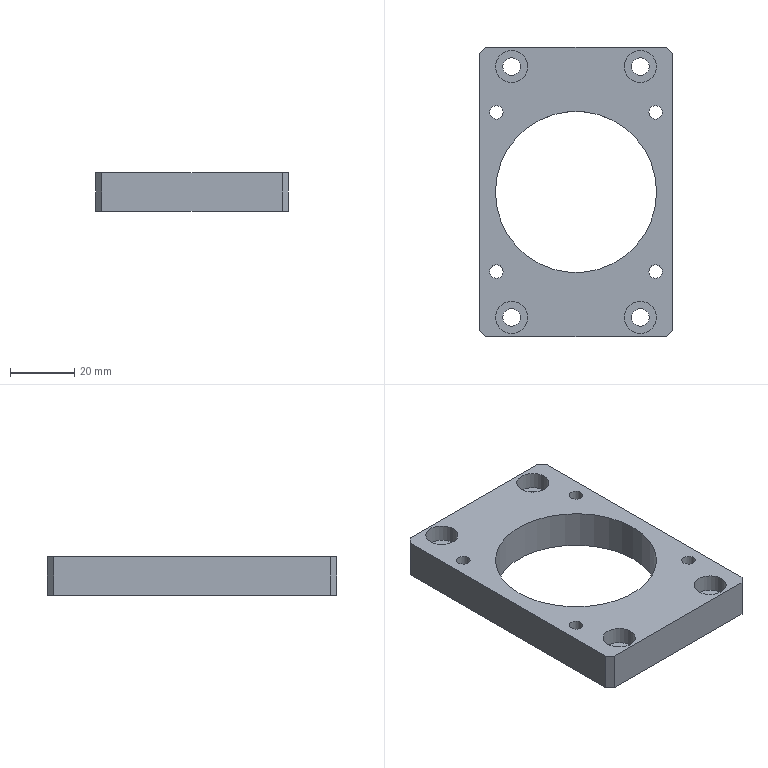Part | NX | 1 solid | 27 faces | box 60 x 90 x 12 mm | volume 38059 mm3 | plane 14 | cylinder 13 | commonest cylinder face diameters 4.2 x4 5.5 x4 10 x4 50.1 x1
STEP:
#1=CARTESIAN_POINT('',(-28.,45.,6.));
#2=VERTEX_POINT('',#1);
#3=CARTESIAN_POINT('',(-30.,43.,6.));
#4=VERTEX_POINT('',#3);
#5=CARTESIAN_POINT('',(-36.5,36.5,6.));
#6=DIRECTION('',(-0.7071,-0.7071,0.));
#7=VECTOR('',#6,1000.);
#8=LINE('',#5,#7);
#9=EDGE_CURVE('',#2,#4,#8,.T.);
#10=ORIENTED_EDGE('',*,*,#9,.F.);
#11=CARTESIAN_POINT('',(-28.,45.,-6.));
#12=VERTEX_POINT('',#11);
#13=CARTESIAN_POINT('',(-28.,45.,6.));
#14=DIRECTION('',(0.,0.,1.));
#15=VECTOR('',#14,1000.);
#16=LINE('',#13,#15);
#17=EDGE_CURVE('',#12,#2,#16,.T.);
#18=ORIENTED_EDGE('',*,*,#17,.F.);
#19=CARTESIAN_POINT('',(-30.,43.,-6.));
#20=VERTEX_POINT('',#19);
#21=CARTESIAN_POINT('',(-30.,43.,-6.));
#22=DIRECTION('',(0.7071,0.7071,0.));
#23=VECTOR('',#22,1000.);
#24=LINE('',#21,#23);
#25=EDGE_CURVE('',#20,#12,#24,.T.);
#26=ORIENTED_EDGE('',*,*,#25,.F.);
#27=CARTESIAN_POINT('',(-30.,43.,6.));
#28=DIRECTION('',(0.,0.,-1.));
#29=VECTOR('',#28,1000.);
#30=LINE('',#27,#29);
#31=EDGE_CURVE('',#4,#20,#30,.T.);
#32=ORIENTED_EDGE('',*,*,#31,.F.);
#33=EDGE_LOOP('',(#10,#18,#26,#32));
#34=FACE_BOUND('',#33,.T.);
#35=CARTESIAN_POINT('',(-30.,43.,6.));
#36=DIRECTION('',(0.7071,-0.7071,0.));
#37=DIRECTION('',(0.,0.,-1.));
#38=AXIS2_PLACEMENT_3D('',#35,#36,#37);
#39=PLANE('',#38);
#40=ADVANCED_FACE('',(#34),#39,.F.);
#41=CARTESIAN_POINT('',(-30.,-43.,6.));
#42=VERTEX_POINT('',#41);
#43=CARTESIAN_POINT('',(-28.,-45.,6.));
#44=VERTEX_POINT('',#43);
#45=CARTESIAN_POINT('',(-36.5,-36.5,6.));
#46=DIRECTION('',(0.7071,-0.7071,0.));
#47=VECTOR('',#46,1000.);
#48=LINE('',#45,#47);
#49=EDGE_CURVE('',#42,#44,#48,.T.);
#50=ORIENTED_EDGE('',*,*,#49,.F.);
#51=CARTESIAN_POINT('',(-30.,-43.,-6.));
#52=VERTEX_POINT('',#51);
#53=CARTESIAN_POINT('',(-30.,-43.,6.));
#54=DIRECTION('',(0.,0.,1.));
#55=VECTOR('',#54,1000.);
#56=LINE('',#53,#55);
#57=EDGE_CURVE('',#52,#42,#56,.T.);
#58=ORIENTED_EDGE('',*,*,#57,.F.);
#59=CARTESIAN_POINT('',(-28.,-45.,-6.));
#60=VERTEX_POINT('',#59);
#61=CARTESIAN_POINT('',(-28.,-45.,-6.));
#62=DIRECTION('',(-0.7071,0.7071,0.));
#63=VECTOR('',#62,1000.);
#64=LINE('',#61,#63);
#65=EDGE_CURVE('',#60,#52,#64,.T.);
#66=ORIENTED_EDGE('',*,*,#65,.F.);
#67=CARTESIAN_POINT('',(-28.,-45.,6.));
#68=DIRECTION('',(0.,0.,-1.));
#69=VECTOR('',#68,1000.);
#70=LINE('',#67,#69);
#71=EDGE_CURVE('',#44,#60,#70,.T.);
#72=ORIENTED_EDGE('',*,*,#71,.F.);
#73=EDGE_LOOP('',(#50,#58,#66,#72));
#74=FACE_BOUND('',#73,.T.);
#75=CARTESIAN_POINT('',(-28.,-45.,6.));
#76=DIRECTION('',(0.7071,0.7071,0.));
#77=DIRECTION('',(0.,0.,-1.));
#78=AXIS2_PLACEMENT_3D('',#75,#76,#77);
#79=PLANE('',#78);
#80=ADVANCED_FACE('',(#74),#79,.F.);
#81=CARTESIAN_POINT('',(28.,-45.,6.));
#82=VERTEX_POINT('',#81);
#83=CARTESIAN_POINT('',(30.,-43.,6.));
#84=VERTEX_POINT('',#83);
#85=CARTESIAN_POINT('',(36.5,-36.5,6.));
#86=DIRECTION('',(0.7071,0.7071,0.));
#87=VECTOR('',#86,1000.);
#88=LINE('',#85,#87);
#89=EDGE_CURVE('',#82,#84,#88,.T.);
#90=ORIENTED_EDGE('',*,*,#89,.F.);
#91=CARTESIAN_POINT('',(28.,-45.,-6.));
#92=VERTEX_POINT('',#91);
#93=CARTESIAN_POINT('',(28.,-45.,6.));
#94=DIRECTION('',(0.,0.,1.));
#95=VECTOR('',#94,1000.);
#96=LINE('',#93,#95);
#97=EDGE_CURVE('',#92,#82,#96,.T.);
#98=ORIENTED_EDGE('',*,*,#97,.F.);
#99=CARTESIAN_POINT('',(30.,-43.,-6.));
#100=VERTEX_POINT('',#99);
#101=CARTESIAN_POINT('',(30.,-43.,-6.));
#102=DIRECTION('',(-0.7071,-0.7071,0.));
#103=VECTOR('',#102,1000.);
#104=LINE('',#101,#103);
#105=EDGE_CURVE('',#100,#92,#104,.T.);
#106=ORIENTED_EDGE('',*,*,#105,.F.);
#107=CARTESIAN_POINT('',(30.,-43.,6.));
#108=DIRECTION('',(0.,0.,-1.));
#109=VECTOR('',#108,1000.);
#110=LINE('',#107,#109);
#111=EDGE_CURVE('',#84,#100,#110,.T.);
#112=ORIENTED_EDGE('',*,*,#111,.F.);
#113=EDGE_LOOP('',(#90,#98,#106,#112));
#114=FACE_BOUND('',#113,.T.);
#115=CARTESIAN_POINT('',(30.,-43.,6.));
#116=DIRECTION('',(-0.7071,0.7071,0.));
#117=DIRECTION('',(0.,0.,-1.));
#118=AXIS2_PLACEMENT_3D('',#115,#116,#117);
#119=PLANE('',#118);
#120=ADVANCED_FACE('',(#114),#119,.F.);
#121=CARTESIAN_POINT('',(30.,43.,6.));
#122=VERTEX_POINT('',#121);
#123=CARTESIAN_POINT('',(28.,45.,6.));
#124=VERTEX_POINT('',#123);
#125=CARTESIAN_POINT('',(36.5,36.5,6.));
#126=DIRECTION('',(-0.7071,0.7071,0.));
#127=VECTOR('',#126,1000.);
#128=LINE('',#125,#127);
#129=EDGE_CURVE('',#122,#124,#128,.T.);
#130=ORIENTED_EDGE('',*,*,#129,.F.);
#131=CARTESIAN_POINT('',(30.,43.,-6.));
#132=VERTEX_POINT('',#131);
#133=CARTESIAN_POINT('',(30.,43.,6.));
#134=DIRECTION('',(0.,0.,1.));
#135=VECTOR('',#134,1000.);
#136=LINE('',#133,#135);
#137=EDGE_CURVE('',#132,#122,#136,.T.);
#138=ORIENTED_EDGE('',*,*,#137,.F.);
#139=CARTESIAN_POINT('',(28.,45.,-6.));
#140=VERTEX_POINT('',#139);
#141=CARTESIAN_POINT('',(28.,45.,-6.));
#142=DIRECTION('',(0.7071,-0.7071,0.));
#143=VECTOR('',#142,1000.);
#144=LINE('',#141,#143);
#145=EDGE_CURVE('',#140,#132,#144,.T.);
#146=ORIENTED_EDGE('',*,*,#145,.F.);
#147=CARTESIAN_POINT('',(28.,45.,6.));
#148=DIRECTION('',(0.,0.,-1.));
#149=VECTOR('',#148,1000.);
#150=LINE('',#147,#149);
#151=EDGE_CURVE('',#124,#140,#150,.T.);
#152=ORIENTED_EDGE('',*,*,#151,.F.);
#153=EDGE_LOOP('',(#130,#138,#146,#152));
#154=FACE_BOUND('',#153,.T.);
#155=CARTESIAN_POINT('',(28.,45.,6.));
#156=DIRECTION('',(-0.7071,-0.7071,0.));
#157=DIRECTION('',(0.,0.,-1.));
#158=AXIS2_PLACEMENT_3D('',#155,#156,#157);
#159=PLANE('',#158);
#160=ADVANCED_FACE('',(#154),#159,.F.);
#161=CARTESIAN_POINT('',(-15.,-39.,0.6));
#162=VERTEX_POINT('',#161);
#163=CARTESIAN_POINT('',(-20.,-39.,0.6));
#164=DIRECTION('',(0.,0.,1.));
#165=DIRECTION('',(1.,0.,0.));
#166=AXIS2_PLACEMENT_3D('',#163,#164,#165);
#167=CIRCLE('',#166,5.);
#168=EDGE_CURVE('',#162,#162,#167,.T.);
#169=ORIENTED_EDGE('',*,*,#168,.T.);
#170=EDGE_LOOP('',(#169));
#171=FACE_BOUND('',#170,.T.);
#172=CARTESIAN_POINT('',(-17.25,-39.,0.6));
#173=VERTEX_POINT('',#172);
#174=CARTESIAN_POINT('',(-20.,-39.,0.6));
#175=DIRECTION('',(0.,0.,1.));
#176=DIRECTION('',(1.,0.,0.));
#177=AXIS2_PLACEMENT_3D('',#174,#175,#176);
#178=CIRCLE('',#177,2.75);
#179=EDGE_CURVE('',#173,#173,#178,.T.);
#180=ORIENTED_EDGE('',*,*,#179,.F.);
#181=EDGE_LOOP('',(#180));
#182=FACE_BOUND('',#181,.T.);
#183=CARTESIAN_POINT('',(-17.25,-39.,0.6));
#184=DIRECTION('',(0.,0.,-1.));
#185=DIRECTION('',(-1.,0.,0.));
#186=AXIS2_PLACEMENT_3D('',#183,#184,#185);
#187=PLANE('',#186);
#188=ADVANCED_FACE('',(#171,#182),#187,.F.);
#189=CARTESIAN_POINT('',(15.,-39.,0.6));
#190=VERTEX_POINT('',#189);
#191=CARTESIAN_POINT('',(20.,-39.,0.6));
#192=DIRECTION('',(0.,0.,1.));
#193=DIRECTION('',(-1.,0.,0.));
#194=AXIS2_PLACEMENT_3D('',#191,#192,#193);
#195=CIRCLE('',#194,5.);
#196=EDGE_CURVE('',#190,#190,#195,.T.);
#197=ORIENTED_EDGE('',*,*,#196,.T.);
#198=EDGE_LOOP('',(#197));
#199=FACE_BOUND('',#198,.T.);
#200=CARTESIAN_POINT('',(17.25,-39.,0.6));
#201=VERTEX_POINT('',#200);
#202=CARTESIAN_POINT('',(20.,-39.,0.6));
#203=DIRECTION('',(0.,0.,1.));
#204=DIRECTION('',(-1.,0.,0.));
#205=AXIS2_PLACEMENT_3D('',#202,#203,#204);
#206=CIRCLE('',#205,2.75);
#207=EDGE_CURVE('',#201,#201,#206,.T.);
#208=ORIENTED_EDGE('',*,*,#207,.F.);
#209=EDGE_LOOP('',(#208));
#210=FACE_BOUND('',#209,.T.);
#211=CARTESIAN_POINT('',(-17.25,-39.,0.6));
#212=DIRECTION('',(0.,0.,-1.));
#213=DIRECTION('',(-1.,0.,0.));
#214=AXIS2_PLACEMENT_3D('',#211,#212,#213);
#215=PLANE('',#214);
#216=ADVANCED_FACE('',(#199,#210),#215,.F.);
#217=CARTESIAN_POINT('',(-25.,39.,0.6));
#218=VERTEX_POINT('',#217);
#219=CARTESIAN_POINT('',(-20.,39.,0.6));
#220=DIRECTION('',(0.,0.,1.));
#221=DIRECTION('',(-1.,0.,0.));
#222=AXIS2_PLACEMENT_3D('',#219,#220,#221);
#223=CIRCLE('',#222,5.);
#224=EDGE_CURVE('',#218,#218,#223,.T.);
#225=ORIENTED_EDGE('',*,*,#224,.T.);
#226=EDGE_LOOP('',(#225));
#227=FACE_BOUND('',#226,.T.);
#228=CARTESIAN_POINT('',(-22.75,39.,0.6));
#229=VERTEX_POINT('',#228);
#230=CARTESIAN_POINT('',(-20.,39.,0.6));
#231=DIRECTION('',(0.,0.,1.));
#232=DIRECTION('',(-1.,0.,0.));
#233=AXIS2_PLACEMENT_3D('',#230,#231,#232);
#234=CIRCLE('',#233,2.75);
#235=EDGE_CURVE('',#229,#229,#234,.T.);
#236=ORIENTED_EDGE('',*,*,#235,.F.);
#237=EDGE_LOOP('',(#236));
#238=FACE_BOUND('',#237,.T.);
#239=CARTESIAN_POINT('',(-17.25,-39.,0.6));
#240=DIRECTION('',(0.,0.,-1.));
#241=DIRECTION('',(-1.,0.,0.));
#242=AXIS2_PLACEMENT_3D('',#239,#240,#241);
#243=PLANE('',#242);
#244=ADVANCED_FACE('',(#227,#238),#243,.F.);
#245=CARTESIAN_POINT('',(15.,39.,0.6));
#246=VERTEX_POINT('',#245);
#247=CARTESIAN_POINT('',(20.,39.,0.6));
#248=DIRECTION('',(0.,0.,1.));
#249=DIRECTION('',(-1.,0.,0.));
#250=AXIS2_PLACEMENT_3D('',#247,#248,#249);
#251=CIRCLE('',#250,5.);
#252=EDGE_CURVE('',#246,#246,#251,.T.);
#253=ORIENTED_EDGE('',*,*,#252,.T.);
#254=EDGE_LOOP('',(#253));
#255=FACE_BOUND('',#254,.T.);
#256=CARTESIAN_POINT('',(17.25,39.,0.6));
#257=VERTEX_POINT('',#256);
#258=CARTESIAN_POINT('',(20.,39.,0.6));
#259=DIRECTION('',(0.,0.,1.));
#260=DIRECTION('',(-1.,0.,0.));
#261=AXIS2_PLACEMENT_3D('',#258,#259,#260);
#262=CIRCLE('',#261,2.75);
#263=EDGE_CURVE('',#257,#257,#262,.T.);
#264=ORIENTED_EDGE('',*,*,#263,.F.);
#265=EDGE_LOOP('',(#264));
#266=FACE_BOUND('',#265,.T.);
#267=CARTESIAN_POINT('',(-17.25,-39.,0.6));
#268=DIRECTION('',(0.,0.,-1.));
#269=DIRECTION('',(-1.,0.,0.));
#270=AXIS2_PLACEMENT_3D('',#267,#268,#269);
#271=PLANE('',#270);
#272=ADVANCED_FACE('',(#255,#266),#271,.F.);
#273=CARTESIAN_POINT('',(30.,45.,-6.));
#274=DIRECTION('',(-1.,0.,0.));
#275=VECTOR('',#274,1000.);
#276=LINE('',#273,#275);
#277=EDGE_CURVE('',#140,#12,#276,.T.);
#278=ORIENTED_EDGE('',*,*,#277,.F.);
#279=ORIENTED_EDGE('',*,*,#145,.T.);
#280=CARTESIAN_POINT('',(30.,-45.,-6.));
#281=DIRECTION('',(0.,1.,0.));
#282=VECTOR('',#281,1000.);
#283=LINE('',#280,#282);
#284=EDGE_CURVE('',#100,#132,#283,.T.);
#285=ORIENTED_EDGE('',*,*,#284,.F.);
#286=ORIENTED_EDGE('',*,*,#105,.T.);
#287=CARTESIAN_POINT('',(30.,-45.,-6.));
#288=DIRECTION('',(1.,0.,0.));
#289=VECTOR('',#288,1000.);
#290=LINE('',#287,#289);
#291=EDGE_CURVE('',#60,#92,#290,.T.);
#292=ORIENTED_EDGE('',*,*,#291,.F.);
#293=ORIENTED_EDGE('',*,*,#65,.T.);
#294=CARTESIAN_POINT('',(-30.,-45.,-6.));
#295=DIRECTION('',(0.,-1.,0.));
#296=VECTOR('',#295,1000.);
#297=LINE('',#294,#296);
#298=EDGE_CURVE('',#20,#52,#297,.T.);
#299=ORIENTED_EDGE('',*,*,#298,.F.);
#300=ORIENTED_EDGE('',*,*,#25,.T.);
#301=EDGE_LOOP('',(#278,#279,#285,#286,#292,#293,#299,#300));
#302=FACE_BOUND('',#301,.T.);
#303=CARTESIAN_POINT('',(26.849,24.749,-6.));
#304=VERTEX_POINT('',#303);
#305=CARTESIAN_POINT('',(24.749,24.749,-6.));
#306=DIRECTION('',(0.,0.,1.));
#307=DIRECTION('',(1.,0.,0.));
#308=AXIS2_PLACEMENT_3D('',#305,#306,#307);
#309=CIRCLE('',#308,2.1);
#310=EDGE_CURVE('',#304,#304,#309,.T.);
#311=ORIENTED_EDGE('',*,*,#310,.T.);
#312=EDGE_LOOP('',(#311));
#313=FACE_BOUND('',#312,.T.);
#314=CARTESIAN_POINT('',(26.849,-24.749,-6.));
#315=VERTEX_POINT('',#314);
#316=CARTESIAN_POINT('',(24.749,-24.749,-6.));
#317=DIRECTION('',(0.,0.,1.));
#318=DIRECTION('',(1.,0.,0.));
#319=AXIS2_PLACEMENT_3D('',#316,#317,#318);
#320=CIRCLE('',#319,2.1);
#321=EDGE_CURVE('',#315,#315,#320,.T.);
#322=ORIENTED_EDGE('',*,*,#321,.T.);
#323=EDGE_LOOP('',(#322));
#324=FACE_BOUND('',#323,.T.);
#325=CARTESIAN_POINT('',(-22.649,-24.749,-6.));
#326=VERTEX_POINT('',#325);
#327=CARTESIAN_POINT('',(-24.749,-24.749,-6.));
#328=DIRECTION('',(0.,0.,1.));
#329=DIRECTION('',(1.,0.,0.));
#330=AXIS2_PLACEMENT_3D('',#327,#328,#329);
#331=CIRCLE('',#330,2.1);
#332=EDGE_CURVE('',#326,#326,#331,.T.);
#333=ORIENTED_EDGE('',*,*,#332,.T.);
#334=EDGE_LOOP('',(#333));
#335=FACE_BOUND('',#334,.T.);
#336=CARTESIAN_POINT('',(-22.649,24.749,-6.));
#337=VERTEX_POINT('',#336);
#338=CARTESIAN_POINT('',(-24.749,24.749,-6.));
#339=DIRECTION('',(0.,0.,1.));
#340=DIRECTION('',(1.,0.,0.));
#341=AXIS2_PLACEMENT_3D('',#338,#339,#340);
#342=CIRCLE('',#341,2.1);
#343=EDGE_CURVE('',#337,#337,#342,.T.);
#344=ORIENTED_EDGE('',*,*,#343,.T.);
#345=EDGE_LOOP('',(#344));
#346=FACE_BOUND('',#345,.T.);
#347=CARTESIAN_POINT('',(25.05,0.,-6.));
#348=VERTEX_POINT('',#347);
#349=CARTESIAN_POINT('',(0.,0.,-6.));
#350=DIRECTION('',(0.,0.,1.));
#351=DIRECTION('',(1.,0.,0.));
#352=AXIS2_PLACEMENT_3D('',#349,#350,#351);
#353=CIRCLE('',#352,25.05);
#354=EDGE_CURVE('',#348,#348,#353,.T.);
#355=ORIENTED_EDGE('',*,*,#354,.T.);
#356=EDGE_LOOP('',(#355));
#357=FACE_BOUND('',#356,.T.);
#358=CARTESIAN_POINT('',(22.75,39.,-6.));
#359=VERTEX_POINT('',#358);
#360=CARTESIAN_POINT('',(20.,39.,-6.));
#361=DIRECTION('',(0.,0.,1.));
#362=DIRECTION('',(1.,0.,0.));
#363=AXIS2_PLACEMENT_3D('',#360,#361,#362);
#364=CIRCLE('',#363,2.75);
#365=EDGE_CURVE('',#359,#359,#364,.T.);
#366=ORIENTED_EDGE('',*,*,#365,.T.);
#367=EDGE_LOOP('',(#366));
#368=FACE_BOUND('',#367,.T.);
#369=CARTESIAN_POINT('',(-17.25,39.,-6.));
#370=VERTEX_POINT('',#369);
#371=CARTESIAN_POINT('',(-20.,39.,-6.));
#372=DIRECTION('',(0.,0.,1.));
#373=DIRECTION('',(1.,0.,0.));
#374=AXIS2_PLACEMENT_3D('',#371,#372,#373);
#375=CIRCLE('',#374,2.75);
#376=EDGE_CURVE('',#370,#370,#375,.T.);
#377=ORIENTED_EDGE('',*,*,#376,.T.);
#378=EDGE_LOOP('',(#377));
#379=FACE_BOUND('',#378,.T.);
#380=CARTESIAN_POINT('',(22.75,-39.,-6.));
#381=VERTEX_POINT('',#380);
#382=CARTESIAN_POINT('',(20.,-39.,-6.));
#383=DIRECTION('',(0.,0.,1.));
#384=DIRECTION('',(1.,0.,0.));
#385=AXIS2_PLACEMENT_3D('',#382,#383,#384);
#386=CIRCLE('',#385,2.75);
#387=EDGE_CURVE('',#381,#381,#386,.T.);
#388=ORIENTED_EDGE('',*,*,#387,.T.);
#389=EDGE_LOOP('',(#388));
#390=FACE_BOUND('',#389,.T.);
#391=CARTESIAN_POINT('',(-17.25,-39.,-6.));
#392=VERTEX_POINT('',#391);
#393=CARTESIAN_POINT('',(-20.,-39.,-6.));
#394=DIRECTION('',(0.,0.,1.));
#395=DIRECTION('',(1.,0.,0.));
#396=AXIS2_PLACEMENT_3D('',#393,#394,#395);
#397=CIRCLE('',#396,2.75);
#398=EDGE_CURVE('',#392,#392,#397,.T.);
#399=ORIENTED_EDGE('',*,*,#398,.T.);
#400=EDGE_LOOP('',(#399));
#401=FACE_BOUND('',#400,.T.);
#402=CARTESIAN_POINT('',(0.,0.,-6.));
#403=DIRECTION('',(0.,0.,1.));
#404=DIRECTION('',(1.,0.,0.));
#405=AXIS2_PLACEMENT_3D('',#402,#403,#404);
#406=PLANE('',#405);
#407=ADVANCED_FACE('',(#302,#313,#324,#335,#346,#357,#368,#379,#390,#401),#406,.F.);
#408=CARTESIAN_POINT('',(30.,-45.,6.));
#409=DIRECTION('',(0.,1.,0.));
#410=VECTOR('',#409,1000.);
#411=LINE('',#408,#410);
#412=EDGE_CURVE('',#84,#122,#411,.T.);
#413=ORIENTED_EDGE('',*,*,#412,.T.);
#414=ORIENTED_EDGE('',*,*,#129,.T.);
#415=CARTESIAN_POINT('',(30.,45.,6.));
#416=DIRECTION('',(-1.,0.,0.));
#417=VECTOR('',#416,1000.);
#418=LINE('',#415,#417);
#419=EDGE_CURVE('',#124,#2,#418,.T.);
#420=ORIENTED_EDGE('',*,*,#419,.T.);
#421=ORIENTED_EDGE('',*,*,#9,.T.);
#422=CARTESIAN_POINT('',(-30.,-45.,6.));
#423=DIRECTION('',(0.,-1.,0.));
#424=VECTOR('',#423,1000.);
#425=LINE('',#422,#424);
#426=EDGE_CURVE('',#4,#42,#425,.T.);
#427=ORIENTED_EDGE('',*,*,#426,.T.);
#428=ORIENTED_EDGE('',*,*,#49,.T.);
#429=CARTESIAN_POINT('',(30.,-45.,6.));
#430=DIRECTION('',(1.,0.,0.));
#431=VECTOR('',#430,1000.);
#432=LINE('',#429,#431);
#433=EDGE_CURVE('',#44,#82,#432,.T.);
#434=ORIENTED_EDGE('',*,*,#433,.T.);
#435=ORIENTED_EDGE('',*,*,#89,.T.);
#436=EDGE_LOOP('',(#413,#414,#420,#421,#427,#428,#434,#435));
#437=FACE_BOUND('',#436,.T.);
#438=CARTESIAN_POINT('',(26.849,24.749,6.));
#439=VERTEX_POINT('',#438);
#440=CARTESIAN_POINT('',(24.749,24.749,6.));
#441=DIRECTION('',(0.,0.,1.));
#442=DIRECTION('',(1.,0.,0.));
#443=AXIS2_PLACEMENT_3D('',#440,#441,#442);
#444=CIRCLE('',#443,2.1);
#445=EDGE_CURVE('',#439,#439,#444,.T.);
#446=ORIENTED_EDGE('',*,*,#445,.F.);
#447=EDGE_LOOP('',(#446));
#448=FACE_BOUND('',#447,.T.);
#449=CARTESIAN_POINT('',(26.849,-24.749,6.));
#450=VERTEX_POINT('',#449);
#451=CARTESIAN_POINT('',(24.749,-24.749,6.));
#452=DIRECTION('',(0.,0.,1.));
#453=DIRECTION('',(1.,0.,0.));
#454=AXIS2_PLACEMENT_3D('',#451,#452,#453);
#455=CIRCLE('',#454,2.1);
#456=EDGE_CURVE('',#450,#450,#455,.T.);
#457=ORIENTED_EDGE('',*,*,#456,.F.);
#458=EDGE_LOOP('',(#457));
#459=FACE_BOUND('',#458,.T.);
#460=CARTESIAN_POINT('',(-22.649,-24.749,6.));
#461=VERTEX_POINT('',#460);
#462=CARTESIAN_POINT('',(-24.749,-24.749,6.));
#463=DIRECTION('',(0.,0.,1.));
#464=DIRECTION('',(1.,0.,0.));
#465=AXIS2_PLACEMENT_3D('',#462,#463,#464);
#466=CIRCLE('',#465,2.1);
#467=EDGE_CURVE('',#461,#461,#466,.T.);
#468=ORIENTED_EDGE('',*,*,#467,.F.);
#469=EDGE_LOOP('',(#468));
#470=FACE_BOUND('',#469,.T.);
#471=CARTESIAN_POINT('',(-22.649,24.749,6.));
#472=VERTEX_POINT('',#471);
#473=CARTESIAN_POINT('',(-24.749,24.749,6.));
#474=DIRECTION('',(0.,0.,1.));
#475=DIRECTION('',(1.,0.,0.));
#476=AXIS2_PLACEMENT_3D('',#473,#474,#475);
#477=CIRCLE('',#476,2.1);
#478=EDGE_CURVE('',#472,#472,#477,.T.);
#479=ORIENTED_EDGE('',*,*,#478,.F.);
#480=EDGE_LOOP('',(#479));
#481=FACE_BOUND('',#480,.T.);
#482=CARTESIAN_POINT('',(25.05,0.,6.));
#483=VERTEX_POINT('',#482);
#484=CARTESIAN_POINT('',(0.,0.,6.));
#485=DIRECTION('',(0.,0.,1.));
#486=DIRECTION('',(1.,0.,0.));
#487=AXIS2_PLACEMENT_3D('',#484,#485,#486);
#488=CIRCLE('',#487,25.05);
#489=EDGE_CURVE('',#483,#483,#488,.T.);
#490=ORIENTED_EDGE('',*,*,#489,.F.);
#491=EDGE_LOOP('',(#490));
#492=FACE_BOUND('',#491,.T.);
#493=CARTESIAN_POINT('',(25.,39.,6.));
#494=VERTEX_POINT('',#493);
#495=CARTESIAN_POINT('',(20.,39.,6.));
#496=DIRECTION('',(0.,0.,1.));
#497=DIRECTION('',(1.,0.,0.));
#498=AXIS2_PLACEMENT_3D('',#495,#496,#497);
#499=CIRCLE('',#498,5.);
#500=EDGE_CURVE('',#494,#494,#499,.T.);
#501=ORIENTED_EDGE('',*,*,#500,.F.);
#502=EDGE_LOOP('',(#501));
#503=FACE_BOUND('',#502,.T.);
#504=CARTESIAN_POINT('',(-15.,39.,6.));
#505=VERTEX_POINT('',#504);
#506=CARTESIAN_POINT('',(-20.,39.,6.));
#507=DIRECTION('',(0.,0.,1.));
#508=DIRECTION('',(1.,0.,0.));
#509=AXIS2_PLACEMENT_3D('',#506,#507,#508);
#510=CIRCLE('',#509,5.);
#511=EDGE_CURVE('',#505,#505,#510,.T.);
#512=ORIENTED_EDGE('',*,*,#511,.F.);
#513=EDGE_LOOP('',(#512));
#514=FACE_BOUND('',#513,.T.);
#515=CARTESIAN_POINT('',(25.,-39.,6.));
#516=VERTEX_POINT('',#515);
#517=CARTESIAN_POINT('',(20.,-39.,6.));
#518=DIRECTION('',(0.,0.,1.));
#519=DIRECTION('',(1.,0.,0.));
#520=AXIS2_PLACEMENT_3D('',#517,#518,#519);
#521=CIRCLE('',#520,5.);
#522=EDGE_CURVE('',#516,#516,#521,.T.);
#523=ORIENTED_EDGE('',*,*,#522,.F.);
#524=EDGE_LOOP('',(#523));
#525=FACE_BOUND('',#524,.T.);
#526=CARTESIAN_POINT('',(-15.,-39.,6.));
#527=VERTEX_POINT('',#526);
#528=CARTESIAN_POINT('',(-20.,-39.,6.));
#529=DIRECTION('',(0.,0.,1.));
#530=DIRECTION('',(1.,0.,0.));
#531=AXIS2_PLACEMENT_3D('',#528,#529,#530);
#532=CIRCLE('',#531,5.);
#533=EDGE_CURVE('',#527,#527,#532,.T.);
#534=ORIENTED_EDGE('',*,*,#533,.F.);
#535=EDGE_LOOP('',(#534));
#536=FACE_BOUND('',#535,.T.);
#537=CARTESIAN_POINT('',(0.,0.,6.));
#538=DIRECTION('',(0.,0.,1.));
#539=DIRECTION('',(1.,0.,0.));
#540=AXIS2_PLACEMENT_3D('',#537,#538,#539);
#541=PLANE('',#540);
#542=ADVANCED_FACE('',(#437,#448,#459,#470,#481,#492,#503,#514,#525,#536),#541,.T.);
#543=ORIENTED_EDGE('',*,*,#419,.F.);
#544=ORIENTED_EDGE('',*,*,#151,.T.);
#545=ORIENTED_EDGE('',*,*,#277,.T.);
#546=ORIENTED_EDGE('',*,*,#17,.T.);
#547=EDGE_LOOP('',(#543,#544,#545,#546));
#548=FACE_BOUND('',#547,.T.);
#549=CARTESIAN_POINT('',(30.,45.,6.));
#550=DIRECTION('',(0.,-1.,0.));
#551=DIRECTION('',(1.,0.,0.));
#552=AXIS2_PLACEMENT_3D('',#549,#550,#551);
#553=PLANE('',#552);
#554=ADVANCED_FACE('',(#548),#553,.F.);
#555=ORIENTED_EDGE('',*,*,#284,.T.);
#556=ORIENTED_EDGE('',*,*,#137,.T.);
#557=ORIENTED_EDGE('',*,*,#412,.F.);
#558=ORIENTED_EDGE('',*,*,#111,.T.);
#559=EDGE_LOOP('',(#555,#556,#557,#558));
#560=FACE_BOUND('',#559,.T.);
#561=CARTESIAN_POINT('',(30.,-45.,6.));
#562=DIRECTION('',(-1.,0.,0.));
#563=DIRECTION('',(0.,-1.,0.));
#564=AXIS2_PLACEMENT_3D('',#561,#562,#563);
#565=PLANE('',#564);
#566=ADVANCED_FACE('',(#560),#565,.F.);
#567=ORIENTED_EDGE('',*,*,#291,.T.);
#568=ORIENTED_EDGE('',*,*,#97,.T.);
#569=ORIENTED_EDGE('',*,*,#433,.F.);
#570=ORIENTED_EDGE('',*,*,#71,.T.);
#571=EDGE_LOOP('',(#567,#568,#569,#570));
#572=FACE_BOUND('',#571,.T.);
#573=CARTESIAN_POINT('',(30.,-45.,6.));
#574=DIRECTION('',(0.,1.,0.));
#575=DIRECTION('',(-1.,0.,0.));
#576=AXIS2_PLACEMENT_3D('',#573,#574,#575);
#577=PLANE('',#576);
#578=ADVANCED_FACE('',(#572),#577,.F.);
#579=ORIENTED_EDGE('',*,*,#298,.T.);
#580=ORIENTED_EDGE('',*,*,#57,.T.);
#581=ORIENTED_EDGE('',*,*,#426,.F.);
#582=ORIENTED_EDGE('',*,*,#31,.T.);
#583=EDGE_LOOP('',(#579,#580,#581,#582));
#584=FACE_BOUND('',#583,.T.);
#585=CARTESIAN_POINT('',(-30.,-45.,6.));
#586=DIRECTION('',(1.,0.,0.));
#587=DIRECTION('',(0.,0.,-1.));
#588=AXIS2_PLACEMENT_3D('',#585,#586,#587);
#589=PLANE('',#588);
#590=ADVANCED_FACE('',(#584),#589,.F.);
#591=ORIENTED_EDGE('',*,*,#310,.F.);
#592=EDGE_LOOP('',(#591));
#593=FACE_BOUND('',#592,.T.);
#594=ORIENTED_EDGE('',*,*,#445,.T.);
#595=EDGE_LOOP('',(#594));
#596=FACE_BOUND('',#595,.T.);
#597=CARTESIAN_POINT('',(24.749,24.749,6.));
#598=DIRECTION('',(0.,0.,1.));
#599=DIRECTION('',(1.,0.,0.));
#600=AXIS2_PLACEMENT_3D('',#597,#598,#599);
#601=CYLINDRICAL_SURFACE('',#600,2.1);
#602=ADVANCED_FACE('',(#593,#596),#601,.F.);
#603=ORIENTED_EDGE('',*,*,#321,.F.);
#604=EDGE_LOOP('',(#603));
#605=FACE_BOUND('',#604,.T.);
#606=ORIENTED_EDGE('',*,*,#456,.T.);
#607=EDGE_LOOP('',(#606));
#608=FACE_BOUND('',#607,.T.);
#609=CARTESIAN_POINT('',(24.749,-24.749,6.));
#610=DIRECTION('',(0.,0.,1.));
#611=DIRECTION('',(1.,0.,0.));
#612=AXIS2_PLACEMENT_3D('',#609,#610,#611);
#613=CYLINDRICAL_SURFACE('',#612,2.1);
#614=ADVANCED_FACE('',(#605,#608),#613,.F.);
#615=ORIENTED_EDGE('',*,*,#332,.F.);
#616=EDGE_LOOP('',(#615));
#617=FACE_BOUND('',#616,.T.);
#618=ORIENTED_EDGE('',*,*,#467,.T.);
#619=EDGE_LOOP('',(#618));
#620=FACE_BOUND('',#619,.T.);
#621=CARTESIAN_POINT('',(-24.749,-24.749,6.));
#622=DIRECTION('',(0.,0.,1.));
#623=DIRECTION('',(1.,0.,0.));
#624=AXIS2_PLACEMENT_3D('',#621,#622,#623);
#625=CYLINDRICAL_SURFACE('',#624,2.1);
#626=ADVANCED_FACE('',(#617,#620),#625,.F.);
#627=ORIENTED_EDGE('',*,*,#343,.F.);
#628=EDGE_LOOP('',(#627));
#629=FACE_BOUND('',#628,.T.);
#630=ORIENTED_EDGE('',*,*,#478,.T.);
#631=EDGE_LOOP('',(#630));
#632=FACE_BOUND('',#631,.T.);
#633=CARTESIAN_POINT('',(-24.749,24.749,6.));
#634=DIRECTION('',(0.,0.,1.));
#635=DIRECTION('',(1.,0.,0.));
#636=AXIS2_PLACEMENT_3D('',#633,#634,#635);
#637=CYLINDRICAL_SURFACE('',#636,2.1);
#638=ADVANCED_FACE('',(#629,#632),#637,.F.);
#639=ORIENTED_EDGE('',*,*,#354,.F.);
#640=EDGE_LOOP('',(#639));
#641=FACE_BOUND('',#640,.T.);
#642=ORIENTED_EDGE('',*,*,#489,.T.);
#643=EDGE_LOOP('',(#642));
#644=FACE_BOUND('',#643,.T.);
#645=CARTESIAN_POINT('',(0.,0.,-6.));
#646=DIRECTION('',(0.,0.,1.));
#647=DIRECTION('',(1.,0.,0.));
#648=AXIS2_PLACEMENT_3D('',#645,#646,#647);
#649=CYLINDRICAL_SURFACE('',#648,25.05);
#650=ADVANCED_FACE('',(#641,#644),#649,.F.);
#651=ORIENTED_EDGE('',*,*,#365,.F.);
#652=EDGE_LOOP('',(#651));
#653=FACE_BOUND('',#652,.T.);
#654=ORIENTED_EDGE('',*,*,#263,.T.);
#655=EDGE_LOOP('',(#654));
#656=FACE_BOUND('',#655,.T.);
#657=CARTESIAN_POINT('',(20.,39.,6.));
#658=DIRECTION('',(0.,0.,1.));
#659=DIRECTION('',(1.,0.,0.));
#660=AXIS2_PLACEMENT_3D('',#657,#658,#659);
#661=CYLINDRICAL_SURFACE('',#660,2.75);
#662=ADVANCED_FACE('',(#653,#656),#661,.F.);
#663=ORIENTED_EDGE('',*,*,#252,.F.);
#664=EDGE_LOOP('',(#663));
#665=FACE_BOUND('',#664,.T.);
#666=ORIENTED_EDGE('',*,*,#500,.T.);
#667=EDGE_LOOP('',(#666));
#668=FACE_BOUND('',#667,.T.);
#669=CARTESIAN_POINT('',(20.,39.,6.));
#670=DIRECTION('',(0.,0.,1.));
#671=DIRECTION('',(1.,0.,0.));
#672=AXIS2_PLACEMENT_3D('',#669,#670,#671);
#673=CYLINDRICAL_SURFACE('',#672,5.);
#674=ADVANCED_FACE('',(#665,#668),#673,.F.);
#675=ORIENTED_EDGE('',*,*,#376,.F.);
#676=EDGE_LOOP('',(#675));
#677=FACE_BOUND('',#676,.T.);
#678=ORIENTED_EDGE('',*,*,#235,.T.);
#679=EDGE_LOOP('',(#678));
#680=FACE_BOUND('',#679,.T.);
#681=CARTESIAN_POINT('',(-20.,39.,6.));
#682=DIRECTION('',(0.,0.,1.));
#683=DIRECTION('',(1.,0.,0.));
#684=AXIS2_PLACEMENT_3D('',#681,#682,#683);
#685=CYLINDRICAL_SURFACE('',#684,2.75);
#686=ADVANCED_FACE('',(#677,#680),#685,.F.);
#687=ORIENTED_EDGE('',*,*,#224,.F.);
#688=EDGE_LOOP('',(#687));
#689=FACE_BOUND('',#688,.T.);
#690=ORIENTED_EDGE('',*,*,#511,.T.);
#691=EDGE_LOOP('',(#690));
#692=FACE_BOUND('',#691,.T.);
#693=CARTESIAN_POINT('',(-20.,39.,6.));
#694=DIRECTION('',(0.,0.,1.));
#695=DIRECTION('',(1.,0.,0.));
#696=AXIS2_PLACEMENT_3D('',#693,#694,#695);
#697=CYLINDRICAL_SURFACE('',#696,5.);
#698=ADVANCED_FACE('',(#689,#692),#697,.F.);
#699=ORIENTED_EDGE('',*,*,#387,.F.);
#700=EDGE_LOOP('',(#699));
#701=FACE_BOUND('',#700,.T.);
#702=ORIENTED_EDGE('',*,*,#207,.T.);
#703=EDGE_LOOP('',(#702));
#704=FACE_BOUND('',#703,.T.);
#705=CARTESIAN_POINT('',(20.,-39.,6.));
#706=DIRECTION('',(0.,0.,1.));
#707=DIRECTION('',(1.,0.,0.));
#708=AXIS2_PLACEMENT_3D('',#705,#706,#707);
#709=CYLINDRICAL_SURFACE('',#708,2.75);
#710=ADVANCED_FACE('',(#701,#704),#709,.F.);
#711=ORIENTED_EDGE('',*,*,#196,.F.);
#712=EDGE_LOOP('',(#711));
#713=FACE_BOUND('',#712,.T.);
#714=ORIENTED_EDGE('',*,*,#522,.T.);
#715=EDGE_LOOP('',(#714));
#716=FACE_BOUND('',#715,.T.);
#717=CARTESIAN_POINT('',(20.,-39.,6.));
#718=DIRECTION('',(0.,0.,1.));
#719=DIRECTION('',(1.,0.,0.));
#720=AXIS2_PLACEMENT_3D('',#717,#718,#719);
#721=CYLINDRICAL_SURFACE('',#720,5.);
#722=ADVANCED_FACE('',(#713,#716),#721,.F.);
#723=ORIENTED_EDGE('',*,*,#398,.F.);
#724=EDGE_LOOP('',(#723));
#725=FACE_BOUND('',#724,.T.);
#726=ORIENTED_EDGE('',*,*,#179,.T.);
#727=EDGE_LOOP('',(#726));
#728=FACE_BOUND('',#727,.T.);
#729=CARTESIAN_POINT('',(-20.,-39.,6.));
#730=DIRECTION('',(0.,0.,1.));
#731=DIRECTION('',(1.,0.,0.));
#732=AXIS2_PLACEMENT_3D('',#729,#730,#731);
#733=CYLINDRICAL_SURFACE('',#732,2.75);
#734=ADVANCED_FACE('',(#725,#728),#733,.F.);
#735=ORIENTED_EDGE('',*,*,#168,.F.);
#736=EDGE_LOOP('',(#735));
#737=FACE_BOUND('',#736,.T.);
#738=ORIENTED_EDGE('',*,*,#533,.T.);
#739=EDGE_LOOP('',(#738));
#740=FACE_BOUND('',#739,.T.);
#741=CARTESIAN_POINT('',(-20.,-39.,6.));
#742=DIRECTION('',(0.,0.,1.));
#743=DIRECTION('',(1.,0.,0.));
#744=AXIS2_PLACEMENT_3D('',#741,#742,#743);
#745=CYLINDRICAL_SURFACE('',#744,5.);
#746=ADVANCED_FACE('',(#737,#740),#745,.F.);
#747=CLOSED_SHELL('',(#40,#80,#120,#160,#188,#216,#244,#272,#407,#542,#554,#566,#578,#590,#602,#614,#626,#638,#650,#662,#674,#686,#698,#710,#722,#734,#746));
#748=MANIFOLD_SOLID_BREP('',#747);
#749=(LENGTH_UNIT()NAMED_UNIT(*)SI_UNIT(.MILLI.,.METRE.));
#750=UNCERTAINTY_MEASURE_WITH_UNIT(LENGTH_MEASURE(0.00001),#749,'','');
#751=(NAMED_UNIT(*)PLANE_ANGLE_UNIT()SI_UNIT($,.RADIAN.));
#752=(NAMED_UNIT(*)SI_UNIT($,.STERADIAN.)SOLID_ANGLE_UNIT());
#753=(GEOMETRIC_REPRESENTATION_CONTEXT(3)GLOBAL_UNCERTAINTY_ASSIGNED_CONTEXT((#750))GLOBAL_UNIT_ASSIGNED_CONTEXT((#749,#751,#752))REPRESENTATION_CONTEXT('',''));
#754=ADVANCED_BREP_SHAPE_REPRESENTATION('',(#748),#753);